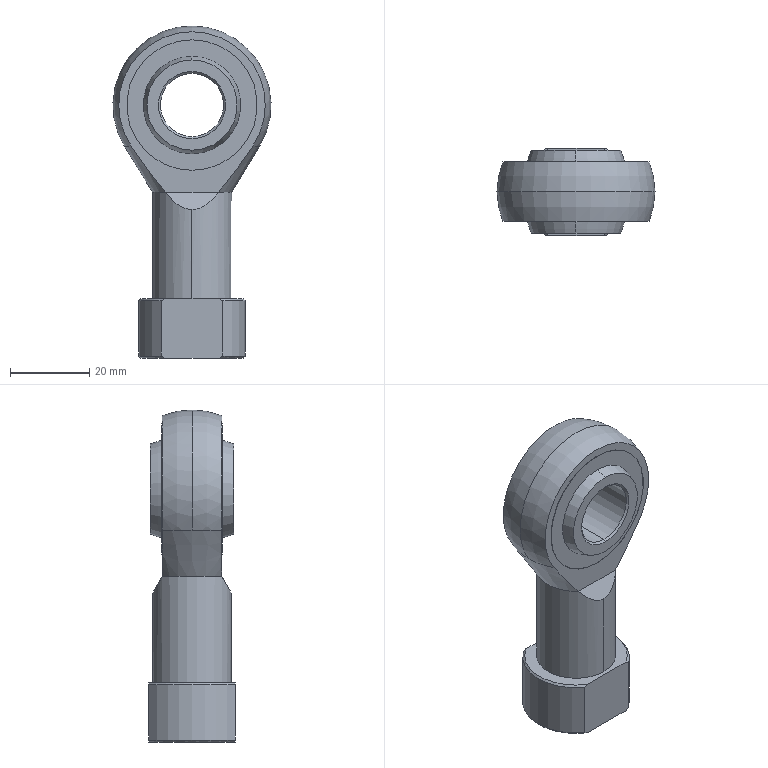Part | STEP file | 1 solid | 45 faces | box 40 x 22 x 84 mm | volume 28902 mm3 | cone 15 | cylinder 12 | plane 12 | other 4 | sphere 2 | commonest cylinder face diameters 33 x4 14.376 x2 16 x2 20 x2 27 x2